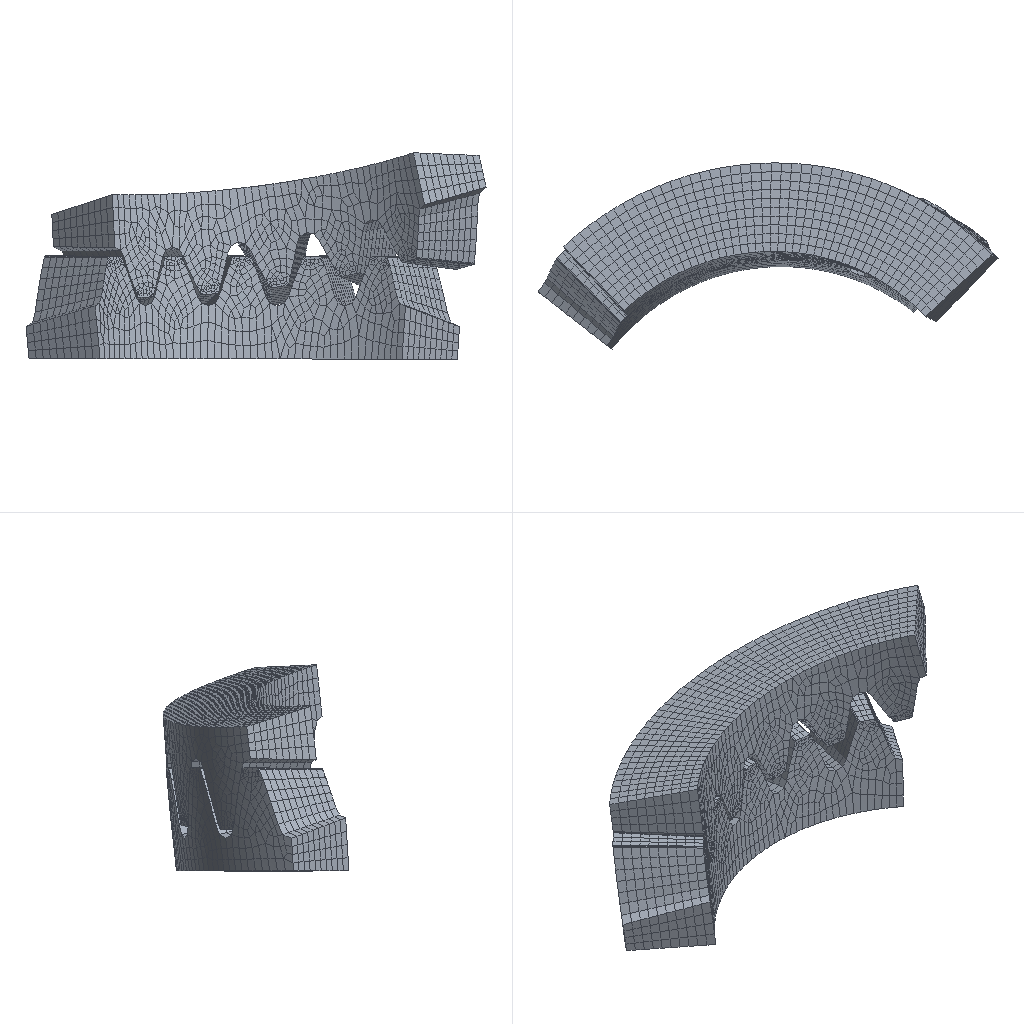Simulation study | abaqus
Set-up summary:
category,name,step,type,value,unit,region
solver,abaqus,,Abaqus/CAE 2024
units,mm-N-s-tonne (MPa),,inferred,E=8900 density=1.38e-09
analysis,contact,,static,nlgeom=True; time_period=1
analysis,load,,static,nlgeom=True; time_period=1
analysis,rotation,,dynamic implicit,nlgeom=True; time_period=1
mesh,nodes,,,11871
mesh,elements,,,9610
element_type,C3D8R,,,8750
element_type,C3D6,,,860
material,peek,,E,8900
material,peek,,nu,0.39
material,peek,,density,1.38e-09
section,peek,,solid section,,,Set-4
section,peek,,solid section,,,Set-3
load,Load-1,load,concentrated moment,"6800 [dir=(0, 0, 1)]",,Set-8
bc,BC-1,contact,fixed,"[dofs=rx,ry,x,y,z n=5]",,Set-9
bc,BC-1,contact,displacement,0.001744 [dofs=rz],,Set-9
bc,BC-2,contact,fixed,"[dofs=rx,ry,rz,x,y,z n=6]",,Set-10
bc,BC-1,load,fixed,"[dofs=rx,ry,x,y,z n=5]",,Set-9
bc,BC-1,load,displacement,0.001744 [dofs=rz],,Set-9
bc,BC-2,load,fixed,"[dofs=rx,ry,x,y,z n=5]",,Set-10
bc,BC-1,rotation,displacement,1.57 [dofs=rz],,Set-9
contact,Int-6,initial,contact pair surface to surface,interaction=IntProp-1; friction=0.04; behavior=hard,,_PickedSurf51 / _PickedSurf50
constraint,coupling,,,2
Abaqus input file, long lists of numbers shortened:
*Heading
** Job name: deck Model name: Model-1
** Generated by: Abaqus/CAE 2024
*Preprint, echo=NO, model=NO, history=NO, contact=NO
**
** PARTS
**
*Part, name=jinggear
*Node
      1,   4.542,    17.026, -0.9307
      2,   4.297,   17.017,  -1.546
** (6125 more lines like these left out)
*Element, type=C3D6
  1,  177,  185,  192,  734,  742,  749
  2,   29,   28,  436,  586,  585,  993
** (508 more lines like these left out)
*Element, type=C3D8R
 511,  156,  158,    6,  157,  713,  715,  563,  714
 512,  153,  152,  159,  154,  710,  709,  716,  711
** (4508 more lines like these left out)
*Nset, nset=Set-4, generate
    1,  6127,     1
*Elset, elset=Set-4, generate
    1,  5020,     1
** Section: Section-1
*Solid Section, elset=Set-4, material=peek
,
*End Part
**
*Part, name=movinggear2
*Node
      1,    16.444,   6.333, -0.9295
      2,   16.293,   6.525,  -1.543
** (5740 more lines like these left out)
*Element, type=C3D6
  1,  184,  191,  198,  706,  713,  720
  2,  183,  198,  190,  705,  720,  712
** (348 more lines like these left out)
*Element, type=C3D8R
 351,  155,  166,    6,    8,  677,  688,  528,  530
 352,  157,  167,  485,  156,  679,  689, 1007,  678
** (4238 more lines like these left out)
*Nset, nset=Set-3, generate
    1,  5742,     1
*Elset, elset=Set-3, generate
    1,  4590,     1
** Section: Section-1
*Solid Section, elset=Set-3, material=peek
,
*End Part
**
**
** ASSEMBLY
**
*Assembly, name=Assembly
**
*Instance, name=jinggear-1, part=jinggear
0.03336, -0.04711, -0.5035
0.03336, -0.04711, -0.5035, 0.5006, 0.8355, -0.5551, 168.331
*End Instance
**
*Instance, name=movinggear2-1, part=movinggear2
-0.000715, -0.0001044, -0.6
-0.000715, -0.0001044, -0.6, 0.00105, -0.001387, 0.4, 115.
*End Instance
**
*Node
      1, -0.003437, 0.004853, -0.2295
*Node
      2, -0.001059, 0.000769, -0.8551
*Nset, nset=Set-8
 2,
*Nset, nset=Set-9
 1,
*Nset, nset=Set-10
 2,
*Nset, nset=m_Set-6
 1,
*Nset, nset=m_Set-7
 2,
*Elset, elset=_m_Surf-13_S5, internal, instance=jinggear-1
   44,   95,  146,  197,  248,  299,  350,  401,  452,  503,  715, 1166, 1617, 2068, 2519, 2970
 3421, 3872, 4323, 4774
*Elset, elset=_m_Surf-13_S4, internal, instance=jinggear-1
  712,  713,  716,  904,  950, 1163, 1164, 1167, 1355, 1401, 1614, 1615, 1618, 1806, 1852, 2065
 2066, 2069, 2257, 2303, 2516, 2517, 2520, 2708, 2754, 2967, 2968, 2971, 3159, 3205, 3418, 3419
** (2 more lines like these left out)
*Elset, elset=_m_Surf-13_S6, internal, instance=jinggear-1
  721,  906, 1172, 1357, 1623, 1808, 2074, 2259, 2525, 2710, 2976, 3161, 3427, 3612, 3878, 4063
 4329, 4514, 4780, 4965
*Surface, type=ELEMENT, name=m_Surf-13
_m_Surf-13_S5, S5
_m_Surf-13_S4, S4
_m_Surf-13_S6, S6
*Elset, elset=_m_Surf-15_S5, internal, instance=jinggear-1, generate
  45,  504,   51
*Elset, elset=_m_Surf-15_S4, internal, instance=jinggear-1
  657,  684,  916, 1108, 1135, 1367, 1559, 1586, 1818, 2010, 2037, 2269, 2461, 2488, 2720, 2912
 2939, 3171, 3363, 3390, 3622, 3814, 3841, 4073, 4265, 4292, 4524, 4716, 4743, 4975
*Elset, elset=_m_Surf-15_S6, internal, instance=jinggear-1
  675,  677,  681, 1126, 1128, 1132, 1577, 1579, 1583, 2028, 2030, 2034, 2479, 2481, 2485, 2930
 2932, 2936, 3381, 3383, 3387, 3832, 3834, 3838, 4283, 4285, 4289, 4734, 4736, 4740
*Elset, elset=_m_Surf-15_S3, internal, instance=jinggear-1
  673,  678, 1124, 1129, 1575, 1580, 2026, 2031, 2477, 2482, 2928, 2933, 3379, 3384, 3830, 3835
 4281, 4286, 4732, 4737
*Surface, type=ELEMENT, name=m_Surf-15
_m_Surf-15_S5, S5
_m_Surf-15_S4, S4
_m_Surf-15_S6, S6
_m_Surf-15_S3, S3
*Elset, elset=_m_Surf-17_S5, internal, instance=jinggear-1
   32,   83,  134,  185,  236,  287,  338,  389,  440,  491,  629,  632, 1080, 1083, 1531, 1534
 1982, 1985, 2433, 2436, 2884, 2887, 3335, 3338, 3786, 3789, 4237, 4240, 4688, 4691
*Elset, elset=_m_Surf-17_S6, internal, instance=jinggear-1
  627,  628,  635, 1078, 1079, 1086, 1529, 1530, 1537, 1980, 1981, 1988, 2431, 2432, 2439, 2882
 2883, 2890, 3333, 3334, 3341, 3784, 3785, 3792, 4235, 4236, 4243, 4686, 4687, 4694
*Elset, elset=_m_Surf-17_S4, internal, instance=jinggear-1
  602,  630, 1053, 1081, 1504, 1532, 1955, 1983, 2406, 2434, 2857, 2885, 3308, 3336, 3759, 3787
 4210, 4238, 4661, 4689
*Elset, elset=_m_Surf-17_S3, internal, instance=jinggear-1, generate
  601,  4660,   451
*Surface, type=ELEMENT, name=m_Surf-17
_m_Surf-17_S5, S5
_m_Surf-17_S6, S6
_m_Surf-17_S4, S4
_m_Surf-17_S3, S3
*Elset, elset=_m_Surf-19_S5, internal, instance=jinggear-1, generate
  31,  490,   51
*Elset, elset=_m_Surf-19_S6, internal, instance=jinggear-1
  555,  568,  570, 1006, 1019, 1021, 1457, 1470, 1472, 1908, 1921, 1923, 2359, 2372, 2374, 2810
 2823, 2825, 3261, 3274, 3276, 3712, 3725, 3727, 4163, 4176, 4178, 4614, 4627, 4629
*Elset, elset=_m_Surf-19_S3, internal, instance=jinggear-1
  556,  582, 1007, 1033, 1458, 1484, 1909, 1935, 2360, 2386, 2811, 2837, 3262, 3288, 3713, 3739
 4164, 4190, 4615, 4641
*Elset, elset=_m_Surf-19_S4, internal, instance=jinggear-1
  567,  583,  851, 1018, 1034, 1302, 1469, 1485, 1753, 1920, 1936, 2204, 2371, 2387, 2655, 2822
 2838, 3106, 3273, 3289, 3557, 3724, 3740, 4008, 4175, 4191, 4459, 4626, 4642, 4910
*Surface, type=ELEMENT, name=m_Surf-19
_m_Surf-19_S5, S5
_m_Surf-19_S6, S6
_m_Surf-19_S4, S4
_m_Surf-19_S3, S3
*Elset, elset=_m_Surf-21_S5, internal, instance=jinggear-1
   42,   93,  144,  195,  246,  297,  348,  399,  450,  501,  917, 1368, 1819, 2270, 2721, 3172
 3623, 4074, 4525, 4976
*Elset, elset=_m_Surf-21_S3, internal, instance=jinggear-1, generate
  516,  4575,   451
*Elset, elset=_m_Surf-21_S4, internal, instance=jinggear-1
  517,  523,  797,  798,  821,  968,  974, 1248, 1249, 1272, 1419, 1425, 1699, 1700, 1723, 1870
 1876, 2150, 2151, 2174, 2321, 2327, 2601, 2602, 2625, 2772, 2778, 3052, 3053, 3076, 3223, 3229
** (2 more lines like these left out)
*Elset, elset=_m_Surf-21_S6, internal, instance=jinggear-1, generate
  544,  4603,   451
*Surface, type=ELEMENT, name=m_Surf-21
_m_Surf-21_S5, S5
_m_Surf-21_S3, S3
_m_Surf-21_S4, S4
_m_Surf-21_S6, S6
*Elset, elset=_s_Surf-13_S3, internal, instance=movinggear2-1
   17,   52,   87,  122,  157,  192,  227,  262,  297,  332,  398,  822, 1246, 1670, 2094, 2518
 2942, 3366, 3790, 4214
*Elset, elset=_s_Surf-13_S6, internal, instance=movinggear2-1
  360,  396,  657,  784,  820, 1081, 1208, 1244, 1505, 1632, 1668, 1929, 2056, 2092, 2353, 2480
 2516, 2777, 2904, 2940, 3201, 3328, 3364, 3625, 3752, 3788, 4049, 4176, 4212, 4473
*Elset, elset=_s_Surf-13_S4, internal, instance=movinggear2-1
  362,  395,  636,  786,  819, 1060, 1210, 1243, 1484, 1634, 1667, 1908, 2058, 2091, 2332, 2482
 2515, 2756, 2906, 2939, 3180, 3330, 3363, 3604, 3754, 3787, 4028, 4178, 4211, 4452
*Elset, elset=_s_Surf-13_S5, internal, instance=movinggear2-1, generate
  393,  4209,   424
*Surface, type=ELEMENT, name=s_Surf-13
_s_Surf-13_S3, S3
_s_Surf-13_S6, S6
_s_Surf-13_S4, S4
_s_Surf-13_S5, S5
*Elset, elset=_s_Surf-15_S3, internal, instance=movinggear2-1
   31,   66,  101,  136,  171,  206,  241,  276,  311,  346,  451,  875, 1299, 1723, 2147, 2571
 2995, 3419, 3843, 4267
*Elset, elset=_s_Surf-15_S6, internal, instance=movinggear2-1
  442,  443,  447,  866,  867,  871, 1290, 1291, 1295, 1714, 1715, 1719, 2138, 2139, 2143, 2562
 2563, 2567, 2986, 2987, 2991, 3410, 3411, 3415, 3834, 3835, 3839, 4258, 4259, 4263
*Elset, elset=_s_Surf-15_S5, internal, instance=movinggear2-1
  440,  444,  448,  864,  868,  872, 1288, 1292, 1296, 1712, 1716, 1720, 2136, 2140, 2144, 2560
 2564, 2568, 2984, 2988, 2992, 3408, 3412, 3416, 3832, 3836, 3840, 4256, 4260, 4264
*Elset, elset=_s_Surf-15_S4, internal, instance=movinggear2-1, generate
  414,  4230,   424
*Surface, type=ELEMENT, name=s_Surf-15
_s_Surf-15_S3, S3
_s_Surf-15_S6, S6
_s_Surf-15_S4, S4
_s_Surf-15_S5, S5
*Elset, elset=_s_Surf-17_S5, internal, instance=movinggear2-1
   27,   62,   97,  132,  167,  202,  237,  272,  307,  342,  485,  909, 1333, 1757, 2181, 2605
 3029, 3453, 3877, 4301
*Elset, elset=_s_Surf-17_S4, internal, instance=movinggear2-1
  468,  484,  486,  490,  892,  908,  910,  914, 1316, 1332, 1334, 1338, 1740, 1756, 1758, 1762
 2164, 2180, 2182, 2186, 2588, 2604, 2606, 2610, 3012, 3028, 3030, 3034, 3436, 3452, 3454, 3458
** (1 more lines like these left out)
*Elset, elset=_s_Surf-17_S6, internal, instance=movinggear2-1
  489,  497,  913,  921, 1337, 1345, 1761, 1769, 2185, 2193, 2609, 2617, 3033, 3041, 3457, 3465
 3881, 3889, 4305, 4313
*Elset, elset=_s_Surf-17_S3, internal, instance=movinggear2-1, generate
  481,  4297,   424
*Surface, type=ELEMENT, name=s_Surf-17
_s_Surf-17_S5, S5
_s_Surf-17_S4, S4
_s_Surf-17_S6, S6
_s_Surf-17_S3, S3
*Elset, elset=_s_Surf-19_S5, internal, instance=movinggear2-1
   23,   58,   93,  128,  163,  198,  233,  268,  303,  338,  547,  971, 1395, 1819, 2243, 2667
 3091, 3515, 3939, 4363
*Elset, elset=_s_Surf-19_S6, internal, instance=movinggear2-1
  543,  545,  967,  969, 1391, 1393, 1815, 1817, 2239, 2241, 2663, 2665, 3087, 3089, 3511, 3513
 3935, 3937, 4359, 4361
*Elset, elset=_s_Surf-19_S4, internal, instance=movinggear2-1
  516,  517,  546,  703,  711,  940,  941,  970, 1127, 1135, 1364, 1365, 1394, 1551, 1559, 1788
 1789, 1818, 1975, 1983, 2212, 2213, 2242, 2399, 2407, 2636, 2637, 2666, 2823, 2831, 3060, 3061
** (2 more lines like these left out)
*Surface, type=ELEMENT, name=s_Surf-19
_s_Surf-19_S5, S5
_s_Surf-19_S6, S6
_s_Surf-19_S4, S4
*Elset, elset=_s_Surf-21_S3, internal, instance=movinggear2-1
  573,  592,  997, 1016, 1421, 1440, 1845, 1864, 2269, 2288, 2693, 2712, 3117, 3136, 3541, 3560
 3965, 3984, 4389, 4408
*Elset, elset=_s_Surf-21_S4, internal, instance=movinggear2-1
  577,  581,  587,  595,  751, 1001, 1005, 1011, 1019, 1175, 1425, 1429, 1435, 1443, 1599, 1849
 1853, 1859, 1867, 2023, 2273, 2277, 2283, 2291, 2447, 2697, 2701, 2707, 2715, 2871, 3121, 3125
** (2 more lines like these left out)
*Elset, elset=_s_Surf-21_S5, internal, instance=movinggear2-1
   28,   63,   98,  133,  168,  203,  238,  273,  308,  343,  566,  990, 1414, 1838, 2262, 2686
 3110, 3534, 3958, 4382
*Surface, type=ELEMENT, name=s_Surf-21
_s_Surf-21_S3, S3
_s_Surf-21_S4, S4
_s_Surf-21_S5, S5
*Elset, elset=_s_Surf-23_S2, internal, instance=jinggear-1
  460,  461,  462,  463,  464,  465,  466,  467,  468,  469,  470,  471,  472,  473,  474,  475
  476,  477,  478,  479,  480,  481,  482,  483,  484,  485,  486,  487,  488,  489,  490,  491
** (30 more lines like these left out)
*Surface, type=ELEMENT, name=s_Surf-23
_s_Surf-23_S2, S2
*Elset, elset=_s_Surf-24_S2, internal, instance=movinggear2-1
  316,  317,  318,  319,  320,  321,  322,  323,  324,  325,  326,  327,  328,  329,  330,  331
  332,  333,  334,  335,  336,  337,  338,  339,  340,  341,  342,  343,  344,  345,  346,  347
** (27 more lines like these left out)
*Surface, type=ELEMENT, name=s_Surf-24
_s_Surf-24_S2, S2
*Elset, elset=__PickedSurf50_S5, internal, instance=jinggear-1
   31,   32,   42,   44,   45,   82,   83,   93,   95,   96,  133,  134,  144,  146,  147,  184
  185,  195,  197,  198,  235,  236,  246,  248,  249,  286,  287,  297,  299,  300,  337,  338
** (17 more lines like these left out)
*Elset, elset=__PickedSurf50_S6, internal, instance=jinggear-1
  537,  539,  540,  544,  555,  560,  568,  570,  581,  622,  627,  628,  635,  652,  653,  663
  675,  677,  681,  721,  732,  906,  907,  909,  988,  990,  991,  995, 1006, 1011, 1019, 1021
** (13 more lines like these left out)
*Elset, elset=__PickedSurf50_S4, internal, instance=jinggear-1
  517,  523,  536,  548,  567,  578,  583,  602,  630,  649,  657,  662,  669,  671,  684,  695
  712,  713,  716,  731,  743,  797,  798,  821,  851,  869,  904,  915,  916,  950,  968,  974
** (17 more lines like these left out)
*Elset, elset=__PickedSurf50_S3, internal, instance=jinggear-1
    2,   28,   33,   53,   79,   84,  104,  130,  135,  155,  181,  186,  206,  232,  237,  257
  283,  288,  308,  334,  339,  359,  385,  390,  410,  436,  441,  461,  487,  492,  516,  526
** (12 more lines like these left out)
*Surface, type=ELEMENT, name=_PickedSurf50, internal
__PickedSurf50_S5, S5
__PickedSurf50_S6, S6
__PickedSurf50_S4, S4
__PickedSurf50_S3, S3
*Elset, elset=__PickedSurf51_S3, internal, instance=movinggear2-1
    3,   15,   16,   17,   22,   31,   38,   50,   51,   52,   57,   66,   73,   85,   86,   87
   92,  101,  108,  120,  121,  122,  127,  136,  143,  155,  156,  157,  162,  171,  178,  190
** (13 more lines like these left out)
*Elset, elset=__PickedSurf51_S5, internal, instance=movinggear2-1
   23,   27,   28,   58,   62,   63,   93,   97,   98,  128,  132,  133,  163,  167,  168,  198
  202,  203,  233,  237,  238,  268,  272,  273,  303,  307,  308,  338,  342,  343,  351,  370
** (18 more lines like these left out)
*Elset, elset=__PickedSurf51_S4, internal, instance=movinggear2-1
  362,  387,  395,  414,  425,  468,  484,  486,  490,  516,  517,  546,  577,  581,  587,  591
  595,  636,  670,  672,  703,  711,  712,  714,  726,  728,  730,  731,  751,  752,  786,  811
** (17 more lines like these left out)
*Elset, elset=__PickedSurf51_S6, internal, instance=movinggear2-1
  360,  396,  438,  442,  443,  447,  465,  466,  489,  497,  528,  535,  538,  543,  545,  590
  657,  695,  696,  784,  820,  862,  866,  867,  871,  889,  890,  913,  921,  952,  959,  962
** (10 more lines like these left out)
*Surface, type=ELEMENT, name=_PickedSurf51, internal
__PickedSurf51_S3, S3
__PickedSurf51_S5, S5
__PickedSurf51_S4, S4
__PickedSurf51_S6, S6
*Nset, nset="_T-jinggear-1-Datum csys-1", internal
Set-9,
*Transform, nset="_T-jinggear-1-Datum csys-1"
0.04295, 0.983, -0.1785, -0.9906, 0.01861, -0.1358
*Nset, nset="_T-movinggear2-1-Datum csys-1", internal
Set-10,
Set-8,
*Transform, nset="_T-movinggear2-1-Datum csys-1"
-0.1219, 0.9925, 0.001488, 0.9925, 0.1219, -0.001596
*Orientation, name="jinggear-1-Datum csys-1"
0.04295, 0.983, -0.1785, -0.9906, 0.01861, -0.1358
1, 0.
*Orientation, name="movinggear2-1-Datum csys-1"
-0.1219, 0.9925, 0.001488, 0.9925, 0.1219, -0.001596
1, 0.
** Constraint: Constraint-1
*Coupling, constraint name=Constraint-1, ref node=m_Set-6, surface=s_Surf-23, orientation="jinggear-1-Datum csys-1"
*Kinematic
** Constraint: Constraint-2
*Coupling, constraint name=Constraint-2, ref node=m_Set-7, surface=s_Surf-24, orientation="movinggear2-1-Datum csys-1"
*Kinematic
*End Assembly
**
** MATERIALS
**
*Material, name=peek
*Density
 1.38e-09,
*Elastic
8900., 0.39
**
** INTERACTION PROPERTIES
**
*Surface Interaction, name=IntProp-1
1.,
*Friction, slip tolerance=0.005
 0.04,
*Surface Behavior, pressure-overclosure=HARD
**
** INTERACTIONS
**
** Interaction: Int-6
*Contact Pair, interaction=IntProp-1, type=SURFACE TO SURFACE
_PickedSurf51, _PickedSurf50
** ----------------------------------------------------------------
**
** STEP: contact
**
*Step, name=contact, nlgeom=YES
*Static
0.1, 1., 1e-05, 0.1
**
** BOUNDARY CONDITIONS
**
** Name: BC-1 Type: Displacement/Rotation
*Boundary
Set-9, 1, 1
Set-9, 2, 2
Set-9, 3, 3
Set-9, 4, 4
Set-9, 5, 5
Set-9, 6, 6, 0.001744
** Name: BC-2 Type: Displacement/Rotation
*Boundary
Set-10, 1, 1
Set-10, 2, 2
Set-10, 3, 3
Set-10, 4, 4
Set-10, 5, 5
Set-10, 6, 6
*Adaptive Mesh Controls, name=Ada-1
1., 0.
**
** OUTPUT REQUESTS
**
*Restart, write, frequency=10
**
** FIELD OUTPUT: F-Output-1
**
*Output, field, variable=PRESELECT
**
** HISTORY OUTPUT: H-Output-1
**
*Output, history, variable=PRESELECT
*End Step
** ----------------------------------------------------------------
**
** STEP: load
**
*Step, name=load, nlgeom=YES
*Static
0.01, 1., 1e-05, 0.1
**
** BOUNDARY CONDITIONS
**
** Name: BC-1 Type: Displacement/Rotation
*Boundary, op=NEW
Set-9, 1, 1
Set-9, 2, 2
Set-9, 3, 3
Set-9, 4, 4
Set-9, 5, 5
Set-9, 6, 6, 0.001744
** Name: BC-2 Type: Displacement/Rotation
*Boundary, op=NEW
Set-10, 1, 1
Set-10, 2, 2
Set-10, 3, 3
Set-10, 4, 4
Set-10, 5, 5
**
** LOADS
**
** Name: Load-1   Type: Moment
*Cload, follower
Set-8, 6, 6800.
**
** OUTPUT REQUESTS
**
*Restart, write, frequency=100
**
** FIELD OUTPUT: F-Output-1
**
*Output, field, variable=PRESELECT
**
** HISTORY OUTPUT: H-Output-1
**
*Output, history, variable=PRESELECT
*End Step
** ----------------------------------------------------------------
**
** STEP: rotation
**
*Step, name=rotation, nlgeom=YES, inc=1000
*Dynamic,application=QUASI-STATIC,initial=NO
0.01,1.,1e-06,0.05
**
** BOUNDARY CONDITIONS
**
** Name: BC-1 Type: Displacement/Rotation
*Boundary
Set-9, 6, 6, 1.57
**
** CONTROLS
**
*Controls, reset
*Controls, parameters=time incrementation
, , , 30, , , , , , ,
**
** OUTPUT REQUESTS
**
*Restart, write, frequency=10000
**
** FIELD OUTPUT: F-Output-1
**
*Output, field, variable=PRESELECT, frequency=1
**
** HISTORY OUTPUT: H-Output-1
**
*Output, history, variable=PRESELECT, frequency=1
*End Step
Results summary:
result,odb.job_status,,,JOB_STATUS_COMPLETED_SUCCESSFULLY,"consistent, unstated (Abaqus has no unit system)"
result,steps[0].procedure,contact,,*STATIC,"consistent, unstated (Abaqus has no unit system)"
result,steps[0].time_period,contact,,1,"consistent, unstated (Abaqus has no unit system)"
result,steps[0].n_frames,contact,,11,"consistent, unstated (Abaqus has no unit system)"
result,steps[0].last_frame.id,contact,,10,"consistent, unstated (Abaqus has no unit system)"
result,steps[0].last_frame.value,contact,,1,"consistent, unstated (Abaqus has no unit system)"
result,steps[0].last_frame.description,contact,,Increment     10: Step Time =    1.000,"consistent, unstated (Abaqus has no unit system)"
result,steps[0].completed,contact,,True,"consistent, unstated (Abaqus has no unit system)"
result,steps[0].max_U_magnitude,contact,,0.03078,"consistent, unstated (Abaqus has no unit system)"
result,steps[0].max_S_mises,contact,,122.65,"consistent, unstated (Abaqus has no unit system)"
result,steps[0].RF_sum[1],contact,,0,"consistent, unstated (Abaqus has no unit system)"
result,steps[0].RF_sum[2],contact,,0,"consistent, unstated (Abaqus has no unit system)"
result,steps[0].RF_sum[3],contact,,0,"consistent, unstated (Abaqus has no unit system)"
result,steps[1].procedure,load,,*STATIC,"consistent, unstated (Abaqus has no unit system)"
result,steps[1].time_period,load,,1,"consistent, unstated (Abaqus has no unit system)"
result,steps[1].n_frames,load,,16,"consistent, unstated (Abaqus has no unit system)"
result,steps[1].last_frame.id,load,,15,"consistent, unstated (Abaqus has no unit system)"
result,steps[1].last_frame.value,load,,1,"consistent, unstated (Abaqus has no unit system)"
result,steps[1].last_frame.description,load,,Increment     15: Step Time =    1.000,"consistent, unstated (Abaqus has no unit system)"
result,steps[1].completed,load,,True,"consistent, unstated (Abaqus has no unit system)"
result,steps[1].max_U_magnitude,load,,0.0509,"consistent, unstated (Abaqus has no unit system)"
result,steps[1].max_S_mises,load,,279.16,"consistent, unstated (Abaqus has no unit system)"
result,steps[1].RF_sum[1],load,,0,"consistent, unstated (Abaqus has no unit system)"
result,steps[1].RF_sum[2],load,,0,"consistent, unstated (Abaqus has no unit system)"
result,steps[1].RF_sum[3],load,,0,"consistent, unstated (Abaqus has no unit system)"
result,steps[2].procedure,rotation,,*DYNAMIC,"consistent, unstated (Abaqus has no unit system)"
result,steps[2].time_period,rotation,,1,"consistent, unstated (Abaqus has no unit system)"
result,steps[2].n_frames,rotation,,36,"consistent, unstated (Abaqus has no unit system)"
result,steps[2].last_frame.id,rotation,,35,"consistent, unstated (Abaqus has no unit system)"
result,steps[2].last_frame.value,rotation,,1,"consistent, unstated (Abaqus has no unit system)"
result,steps[2].last_frame.description,rotation,,Increment     35: Step Time =    1.000,"consistent, unstated (Abaqus has no unit system)"
result,steps[2].completed,rotation,,True,"consistent, unstated (Abaqus has no unit system)"
result,steps[2].max_U_magnitude,rotation,,25.019,"consistent, unstated (Abaqus has no unit system)"
result,steps[2].max_S_mises,rotation,,447.896,"consistent, unstated (Abaqus has no unit system)"
result,steps[2].RF_sum[1],rotation,,0.002502,"consistent, unstated (Abaqus has no unit system)"
result,steps[2].RF_sum[2],rotation,,0.00351,"consistent, unstated (Abaqus has no unit system)"
result,steps[2].RF_sum[3],rotation,,-0.0002289,"consistent, unstated (Abaqus has no unit system)"